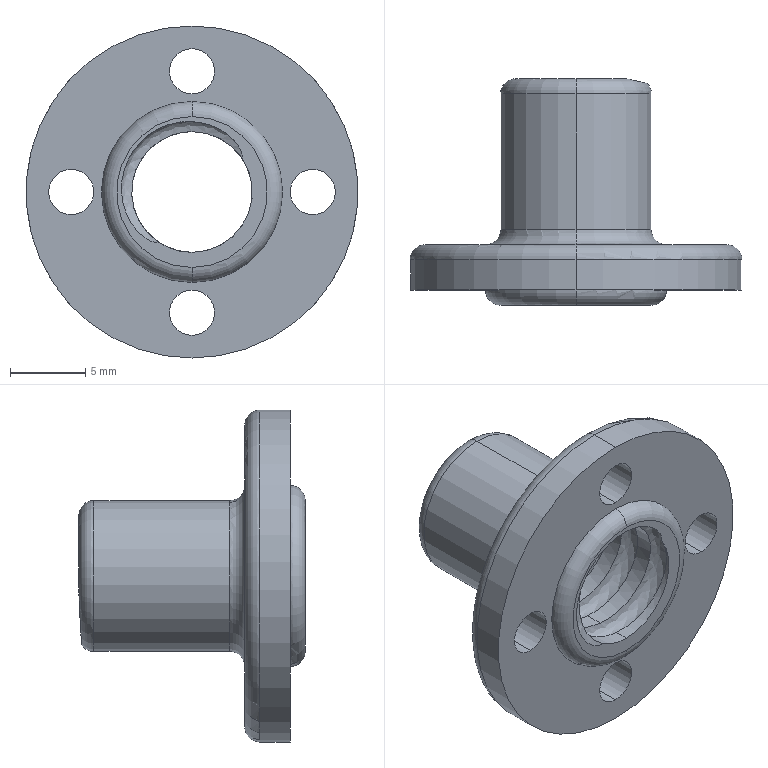Part | STEP file | Lead screw nut 8 | 1 solid | 37 faces | box 22 x 15 x 22 mm | volume 1124 mm3 | cylinder 25 | torus 8 | plane 3 | spline 1 | commonest cylinder face diameters 8 x13 3 x8 10 x2 22 x2